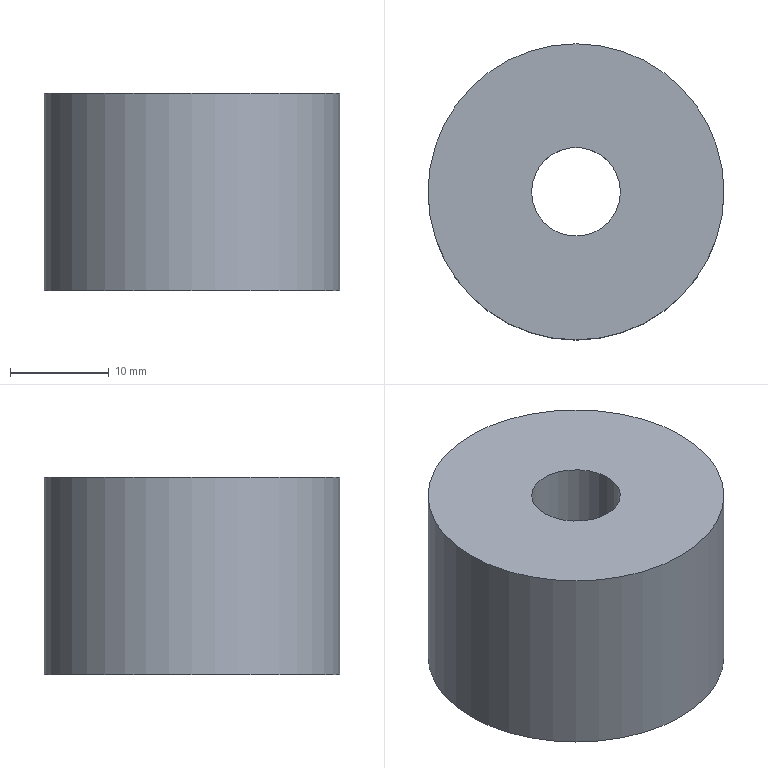Part | STEP file | lll_id94_x_t | 1 solid | 6 faces | box 30 x 30 x 20 mm | volume 11962 mm3 | plane 3 | cylinder 3 | commonest cylinder face diameters 9 x1 14 x1 30 x1
STEP:
#1=CARTESIAN_POINT('',(87.,40.,100.5));
#2=VERTEX_POINT('',#1);
#3=CARTESIAN_POINT('',(80.,40.,100.5));
#4=DIRECTION('',(0.,0.,1.));
#5=DIRECTION('',(1.,0.,0.));
#6=AXIS2_PLACEMENT_3D('',#3,#4,#5);
#7=CIRCLE('',#6,7.);
#8=EDGE_CURVE('',#2,#2,#7,.T.);
#9=ORIENTED_EDGE('',*,*,#8,.T.);
#10=EDGE_LOOP('',(#9));
#11=FACE_BOUND('',#10,.T.);
#12=CARTESIAN_POINT('',(95.,40.,100.5));
#13=VERTEX_POINT('',#12);
#14=CARTESIAN_POINT('',(80.,40.,100.5));
#15=DIRECTION('',(0.,0.,1.));
#16=DIRECTION('',(1.,0.,0.));
#17=AXIS2_PLACEMENT_3D('',#14,#15,#16);
#18=CIRCLE('',#17,15.);
#19=EDGE_CURVE('',#13,#13,#18,.T.);
#20=ORIENTED_EDGE('',*,*,#19,.F.);
#21=EDGE_LOOP('',(#20));
#22=FACE_BOUND('',#21,.T.);
#23=CARTESIAN_POINT('',(0.,0.,100.5));
#24=DIRECTION('',(0.,0.,1.));
#25=DIRECTION('',(1.,0.,0.));
#26=AXIS2_PLACEMENT_3D('',#23,#24,#25);
#27=PLANE('',#26);
#28=ADVANCED_FACE('',(#11,#22),#27,.F.);
#29=CARTESIAN_POINT('',(84.5,40.,120.5));
#30=VERTEX_POINT('',#29);
#31=CARTESIAN_POINT('',(80.,40.,120.5));
#32=DIRECTION('',(0.,0.,1.));
#33=DIRECTION('',(1.,0.,0.));
#34=AXIS2_PLACEMENT_3D('',#31,#32,#33);
#35=CIRCLE('',#34,4.5);
#36=EDGE_CURVE('',#30,#30,#35,.T.);
#37=ORIENTED_EDGE('',*,*,#36,.F.);
#38=EDGE_LOOP('',(#37));
#39=FACE_BOUND('',#38,.T.);
#40=CARTESIAN_POINT('',(65.,40.,120.5));
#41=VERTEX_POINT('',#40);
#42=CARTESIAN_POINT('',(80.,40.,120.5));
#43=DIRECTION('',(0.,0.,-1.));
#44=DIRECTION('',(-1.,0.,0.));
#45=AXIS2_PLACEMENT_3D('',#42,#43,#44);
#46=CIRCLE('',#45,15.);
#47=EDGE_CURVE('',#41,#41,#46,.T.);
#48=ORIENTED_EDGE('',*,*,#47,.F.);
#49=EDGE_LOOP('',(#48));
#50=FACE_BOUND('',#49,.T.);
#51=CARTESIAN_POINT('',(80.,40.,120.5));
#52=DIRECTION('',(0.,0.,1.));
#53=DIRECTION('',(1.,0.,0.));
#54=AXIS2_PLACEMENT_3D('',#51,#52,#53);
#55=PLANE('',#54);
#56=ADVANCED_FACE('',(#39,#50),#55,.T.);
#57=ORIENTED_EDGE('',*,*,#19,.T.);
#58=EDGE_LOOP('',(#57));
#59=FACE_BOUND('',#58,.T.);
#60=ORIENTED_EDGE('',*,*,#47,.T.);
#61=EDGE_LOOP('',(#60));
#62=FACE_BOUND('',#61,.T.);
#63=CARTESIAN_POINT('',(80.,40.,120.5));
#64=DIRECTION('',(0.,0.,-1.));
#65=DIRECTION('',(-1.,0.,0.));
#66=AXIS2_PLACEMENT_3D('',#63,#64,#65);
#67=CYLINDRICAL_SURFACE('',#66,15.);
#68=ADVANCED_FACE('',(#59,#62),#67,.T.);
#69=ORIENTED_EDGE('',*,*,#36,.T.);
#70=EDGE_LOOP('',(#69));
#71=FACE_BOUND('',#70,.T.);
#72=CARTESIAN_POINT('',(84.5,40.,110.5));
#73=VERTEX_POINT('',#72);
#74=CARTESIAN_POINT('',(80.,40.,110.5));
#75=DIRECTION('',(0.,0.,1.));
#76=DIRECTION('',(1.,0.,0.));
#77=AXIS2_PLACEMENT_3D('',#74,#75,#76);
#78=CIRCLE('',#77,4.5);
#79=EDGE_CURVE('',#73,#73,#78,.T.);
#80=ORIENTED_EDGE('',*,*,#79,.F.);
#81=EDGE_LOOP('',(#80));
#82=FACE_BOUND('',#81,.T.);
#83=CARTESIAN_POINT('',(80.,40.,142.5));
#84=DIRECTION('',(0.,0.,1.));
#85=DIRECTION('',(1.,0.,0.));
#86=AXIS2_PLACEMENT_3D('',#83,#84,#85);
#87=CYLINDRICAL_SURFACE('',#86,4.5);
#88=ADVANCED_FACE('',(#71,#82),#87,.F.);
#89=ORIENTED_EDGE('',*,*,#79,.T.);
#90=EDGE_LOOP('',(#89));
#91=FACE_BOUND('',#90,.T.);
#92=CARTESIAN_POINT('',(87.,40.,110.5));
#93=VERTEX_POINT('',#92);
#94=CARTESIAN_POINT('',(80.,40.,110.5));
#95=DIRECTION('',(0.,0.,1.));
#96=DIRECTION('',(1.,0.,0.));
#97=AXIS2_PLACEMENT_3D('',#94,#95,#96);
#98=CIRCLE('',#97,7.);
#99=EDGE_CURVE('',#93,#93,#98,.T.);
#100=ORIENTED_EDGE('',*,*,#99,.F.);
#101=EDGE_LOOP('',(#100));
#102=FACE_BOUND('',#101,.T.);
#103=CARTESIAN_POINT('',(0.,0.,110.5));
#104=DIRECTION('',(0.,0.,1.));
#105=DIRECTION('',(1.,0.,0.));
#106=AXIS2_PLACEMENT_3D('',#103,#104,#105);
#107=PLANE('',#106);
#108=ADVANCED_FACE('',(#91,#102),#107,.F.);
#109=ORIENTED_EDGE('',*,*,#99,.T.);
#110=EDGE_LOOP('',(#109));
#111=FACE_BOUND('',#110,.T.);
#112=ORIENTED_EDGE('',*,*,#8,.F.);
#113=EDGE_LOOP('',(#112));
#114=FACE_BOUND('',#113,.T.);
#115=CARTESIAN_POINT('',(80.,40.,92.5));
#116=DIRECTION('',(0.,0.,1.));
#117=DIRECTION('',(1.,0.,0.));
#118=AXIS2_PLACEMENT_3D('',#115,#116,#117);
#119=CYLINDRICAL_SURFACE('',#118,7.);
#120=ADVANCED_FACE('',(#111,#114),#119,.F.);
#121=CLOSED_SHELL('',(#28,#56,#68,#88,#108,#120));
#122=MANIFOLD_SOLID_BREP('',#121);
#123=(LENGTH_UNIT()NAMED_UNIT(*)SI_UNIT(.MILLI.,.METRE.));
#124=UNCERTAINTY_MEASURE_WITH_UNIT(LENGTH_MEASURE(0.00002),#123,'','');
#125=(NAMED_UNIT(*)PLANE_ANGLE_UNIT()SI_UNIT($,.RADIAN.));
#126=PLANE_ANGLE_MEASURE_WITH_UNIT(PLANE_ANGLE_MEASURE(0.01745),#125);
#127=DIMENSIONAL_EXPONENTS(0.,0.,0.,0.,0.,0.,0.);
#128=(CONVERSION_BASED_UNIT('DEGREE',#126)NAMED_UNIT(#127)PLANE_ANGLE_UNIT());
#129=(NAMED_UNIT(*)SI_UNIT($,.STERADIAN.)SOLID_ANGLE_UNIT());
#130=(GEOMETRIC_REPRESENTATION_CONTEXT(3)GLOBAL_UNCERTAINTY_ASSIGNED_CONTEXT((#124))GLOBAL_UNIT_ASSIGNED_CONTEXT((#123,#128,#129))REPRESENTATION_CONTEXT('',''));
#131=ADVANCED_BREP_SHAPE_REPRESENTATION('',(#122),#130);